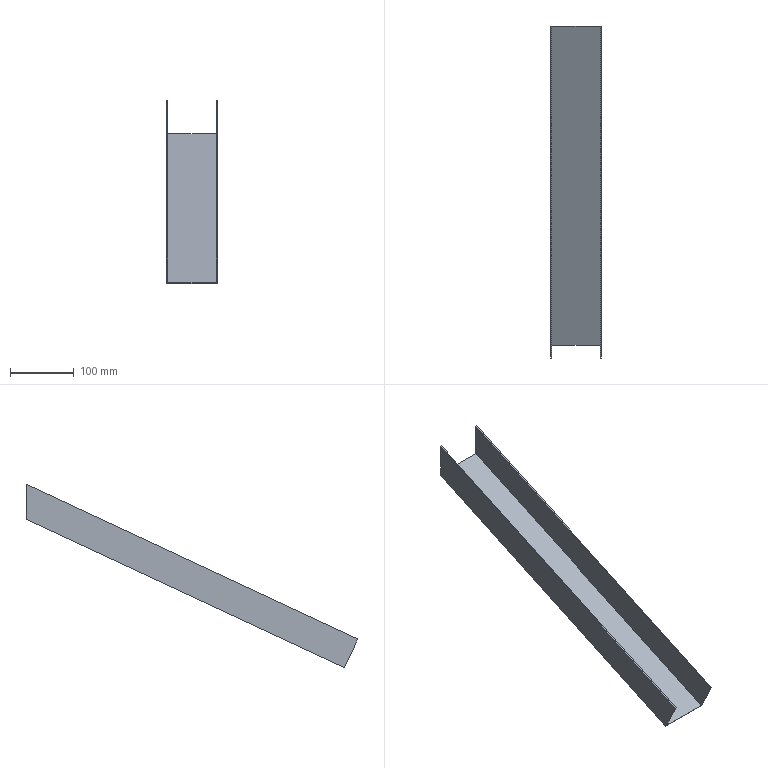Part | NX | features solid 2 | 1 solid | 10 faces | box 80 x 521.131 x 288.323 mm | volume 196597 mm3 | plane 10
STEP:
#1=CARTESIAN_POINT('',(400.,-525.,-154.948));
#2=VERTEX_POINT('',#1);
#3=CARTESIAN_POINT('',(402.,-525.,-154.948));
#4=VERTEX_POINT('',#3);
#5=CARTESIAN_POINT('',(400.,-525.,-154.948));
#6=DIRECTION('',(1.,0.,0.));
#7=VECTOR('',#6,1000.);
#8=LINE('',#5,#7);
#9=EDGE_CURVE('',#2,#4,#8,.T.);
#10=ORIENTED_EDGE('',*,*,#9,.T.);
#11=CARTESIAN_POINT('',(402.,-525.,-207.91));
#12=VERTEX_POINT('',#11);
#13=CARTESIAN_POINT('',(402.,-525.,-175.106));
#14=DIRECTION('',(0.,0.,-1.));
#15=VECTOR('',#14,1000.);
#16=LINE('',#13,#15);
#17=EDGE_CURVE('',#4,#12,#16,.T.);
#18=ORIENTED_EDGE('',*,*,#17,.T.);
#19=CARTESIAN_POINT('',(478.,-525.,-207.91));
#20=VERTEX_POINT('',#19);
#21=CARTESIAN_POINT('',(400.,-525.,-207.91));
#22=DIRECTION('',(1.,0.,0.));
#23=VECTOR('',#22,1000.);
#24=LINE('',#21,#23);
#25=EDGE_CURVE('',#12,#20,#24,.T.);
#26=ORIENTED_EDGE('',*,*,#25,.T.);
#27=CARTESIAN_POINT('',(478.,-525.,-154.948));
#28=VERTEX_POINT('',#27);
#29=CARTESIAN_POINT('',(478.,-525.,-215.));
#30=DIRECTION('',(0.,0.,-1.));
#31=VECTOR('',#30,1000.);
#32=LINE('',#29,#31);
#33=EDGE_CURVE('',#28,#20,#32,.T.);
#34=ORIENTED_EDGE('',*,*,#33,.F.);
#35=CARTESIAN_POINT('',(480.,-525.,-154.948));
#36=VERTEX_POINT('',#35);
#37=CARTESIAN_POINT('',(400.,-525.,-154.948));
#38=DIRECTION('',(1.,0.,0.));
#39=VECTOR('',#38,1000.);
#40=LINE('',#37,#39);
#41=EDGE_CURVE('',#28,#36,#40,.T.);
#42=ORIENTED_EDGE('',*,*,#41,.T.);
#43=CARTESIAN_POINT('',(480.,-525.,-210.116));
#44=VERTEX_POINT('',#43);
#45=CARTESIAN_POINT('',(480.,-525.,-215.));
#46=DIRECTION('',(0.,0.,-1.));
#47=VECTOR('',#46,1000.);
#48=LINE('',#45,#47);
#49=EDGE_CURVE('',#36,#44,#48,.T.);
#50=ORIENTED_EDGE('',*,*,#49,.T.);
#51=CARTESIAN_POINT('',(400.,-525.,-210.116));
#52=VERTEX_POINT('',#51);
#53=CARTESIAN_POINT('',(400.,-525.,-210.116));
#54=DIRECTION('',(1.,0.,0.));
#55=VECTOR('',#54,1000.);
#56=LINE('',#53,#55);
#57=EDGE_CURVE('',#52,#44,#56,.T.);
#58=ORIENTED_EDGE('',*,*,#57,.F.);
#59=CARTESIAN_POINT('',(400.,-525.,-175.106));
#60=DIRECTION('',(0.,0.,-1.));
#61=VECTOR('',#60,1000.);
#62=LINE('',#59,#61);
#63=EDGE_CURVE('',#2,#52,#62,.T.);
#64=ORIENTED_EDGE('',*,*,#63,.F.);
#65=EDGE_LOOP('',(#10,#18,#26,#34,#42,#50,#58,#64));
#66=FACE_BOUND('',#65,.T.);
#67=CARTESIAN_POINT('',(-1120.,-525.,-215.));
#68=DIRECTION('',(0.,1.,0.));
#69=DIRECTION('',(-1.,0.,0.));
#70=AXIS2_PLACEMENT_3D('',#67,#68,#69);
#71=PLANE('',#70);
#72=ADVANCED_FACE('',(#66),#71,.T.);
#73=CARTESIAN_POINT('',(480.,-1046.131,-397.955));
#74=VERTEX_POINT('',#73);
#75=CARTESIAN_POINT('',(478.,-1046.131,-397.955));
#76=VERTEX_POINT('',#75);
#77=CARTESIAN_POINT('',(400.,-1046.131,-397.955));
#78=DIRECTION('',(-1.,0.,0.));
#79=VECTOR('',#78,1000.);
#80=LINE('',#77,#79);
#81=EDGE_CURVE('',#74,#76,#80,.T.);
#82=ORIENTED_EDGE('',*,*,#81,.T.);
#83=CARTESIAN_POINT('',(478.,-1025.845,-441.458));
#84=VERTEX_POINT('',#83);
#85=CARTESIAN_POINT('',(478.,-1046.131,-397.955));
#86=DIRECTION('',(0.,0.4226,-0.9063));
#87=VECTOR('',#86,1000.);
#88=LINE('',#85,#87);
#89=EDGE_CURVE('',#76,#84,#88,.T.);
#90=ORIENTED_EDGE('',*,*,#89,.T.);
#91=CARTESIAN_POINT('',(402.,-1025.845,-441.458));
#92=VERTEX_POINT('',#91);
#93=CARTESIAN_POINT('',(400.,-1025.845,-441.458));
#94=DIRECTION('',(-1.,0.,0.));
#95=VECTOR('',#94,1000.);
#96=LINE('',#93,#95);
#97=EDGE_CURVE('',#84,#92,#96,.T.);
#98=ORIENTED_EDGE('',*,*,#97,.T.);
#99=CARTESIAN_POINT('',(402.,-1046.131,-397.955));
#100=VERTEX_POINT('',#99);
#101=CARTESIAN_POINT('',(402.,-1046.131,-397.955));
#102=DIRECTION('',(0.,0.4226,-0.9063));
#103=VECTOR('',#102,1000.);
#104=LINE('',#101,#103);
#105=EDGE_CURVE('',#100,#92,#104,.T.);
#106=ORIENTED_EDGE('',*,*,#105,.F.);
#107=CARTESIAN_POINT('',(400.,-1046.131,-397.955));
#108=VERTEX_POINT('',#107);
#109=CARTESIAN_POINT('',(400.,-1046.131,-397.955));
#110=DIRECTION('',(-1.,0.,0.));
#111=VECTOR('',#110,1000.);
#112=LINE('',#109,#111);
#113=EDGE_CURVE('',#100,#108,#112,.T.);
#114=ORIENTED_EDGE('',*,*,#113,.T.);
#115=CARTESIAN_POINT('',(400.,-1025.,-443.27));
#116=VERTEX_POINT('',#115);
#117=CARTESIAN_POINT('',(400.,-1046.131,-397.955));
#118=DIRECTION('',(0.,0.4226,-0.9063));
#119=VECTOR('',#118,1000.);
#120=LINE('',#117,#119);
#121=EDGE_CURVE('',#108,#116,#120,.T.);
#122=ORIENTED_EDGE('',*,*,#121,.T.);
#123=CARTESIAN_POINT('',(480.,-1025.,-443.27));
#124=VERTEX_POINT('',#123);
#125=CARTESIAN_POINT('',(400.,-1025.,-443.27));
#126=DIRECTION('',(-1.,0.,0.));
#127=VECTOR('',#126,1000.);
#128=LINE('',#125,#127);
#129=EDGE_CURVE('',#124,#116,#128,.T.);
#130=ORIENTED_EDGE('',*,*,#129,.F.);
#131=CARTESIAN_POINT('',(480.,-1046.131,-397.955));
#132=DIRECTION('',(0.,0.4226,-0.9063));
#133=VECTOR('',#132,1000.);
#134=LINE('',#131,#133);
#135=EDGE_CURVE('',#74,#124,#134,.T.);
#136=ORIENTED_EDGE('',*,*,#135,.F.);
#137=EDGE_LOOP('',(#82,#90,#98,#106,#114,#122,#130,#136));
#138=FACE_BOUND('',#137,.T.);
#139=CARTESIAN_POINT('',(400.,-1046.131,-397.955));
#140=DIRECTION('',(0.,-0.9063,-0.4226));
#141=DIRECTION('',(0.,0.4226,-0.9063));
#142=AXIS2_PLACEMENT_3D('',#139,#140,#141);
#143=PLANE('',#142);
#144=ADVANCED_FACE('',(#138),#143,.T.);
#145=ORIENTED_EDGE('',*,*,#113,.F.);
#146=CARTESIAN_POINT('',(402.,-568.231,-175.106));
#147=DIRECTION('',(0.,0.9063,0.4226));
#148=VECTOR('',#147,1000.);
#149=LINE('',#146,#148);
#150=EDGE_CURVE('',#100,#4,#149,.T.);
#151=ORIENTED_EDGE('',*,*,#150,.T.);
#152=ORIENTED_EDGE('',*,*,#9,.F.);
#153=CARTESIAN_POINT('',(400.,-568.231,-175.106));
#154=DIRECTION('',(0.,0.9063,0.4226));
#155=VECTOR('',#154,1000.);
#156=LINE('',#153,#155);
#157=EDGE_CURVE('',#108,#2,#156,.T.);
#158=ORIENTED_EDGE('',*,*,#157,.F.);
#159=EDGE_LOOP('',(#145,#151,#152,#158));
#160=FACE_BOUND('',#159,.T.);
#161=CARTESIAN_POINT('',(400.,-568.231,-175.106));
#162=DIRECTION('',(0.,0.4226,-0.9063));
#163=DIRECTION('',(-1.,0.,0.));
#164=AXIS2_PLACEMENT_3D('',#161,#162,#163);
#165=PLANE('',#164);
#166=ADVANCED_FACE('',(#160),#165,.F.);
#167=CARTESIAN_POINT('',(400.,-547.1,-220.422));
#168=DIRECTION('',(0.,0.9063,0.4226));
#169=VECTOR('',#168,1000.);
#170=LINE('',#167,#169);
#171=EDGE_CURVE('',#116,#52,#170,.T.);
#172=ORIENTED_EDGE('',*,*,#171,.F.);
#173=ORIENTED_EDGE('',*,*,#121,.F.);
#174=ORIENTED_EDGE('',*,*,#157,.T.);
#175=ORIENTED_EDGE('',*,*,#63,.T.);
#176=EDGE_LOOP('',(#172,#173,#174,#175));
#177=FACE_BOUND('',#176,.T.);
#178=CARTESIAN_POINT('',(400.,-568.231,-175.106));
#179=DIRECTION('',(-1.,0.,0.));
#180=DIRECTION('',(0.,0.,1.));
#181=AXIS2_PLACEMENT_3D('',#178,#179,#180);
#182=PLANE('',#181);
#183=ADVANCED_FACE('',(#177),#182,.T.);
#184=CARTESIAN_POINT('',(480.,-547.1,-220.422));
#185=DIRECTION('',(0.,-0.9063,-0.4226));
#186=VECTOR('',#185,1000.);
#187=LINE('',#184,#186);
#188=EDGE_CURVE('',#44,#124,#187,.T.);
#189=ORIENTED_EDGE('',*,*,#188,.F.);
#190=ORIENTED_EDGE('',*,*,#49,.F.);
#191=CARTESIAN_POINT('',(480.,-568.231,-175.106));
#192=DIRECTION('',(0.,-0.9063,-0.4226));
#193=VECTOR('',#192,1000.);
#194=LINE('',#191,#193);
#195=EDGE_CURVE('',#36,#74,#194,.T.);
#196=ORIENTED_EDGE('',*,*,#195,.T.);
#197=ORIENTED_EDGE('',*,*,#135,.T.);
#198=EDGE_LOOP('',(#189,#190,#196,#197));
#199=FACE_BOUND('',#198,.T.);
#200=CARTESIAN_POINT('',(480.,-568.231,-175.106));
#201=DIRECTION('',(1.,0.,0.));
#202=DIRECTION('',(0.,0.,-1.));
#203=AXIS2_PLACEMENT_3D('',#200,#201,#202);
#204=PLANE('',#203);
#205=ADVANCED_FACE('',(#199),#204,.T.);
#206=ORIENTED_EDGE('',*,*,#41,.F.);
#207=CARTESIAN_POINT('',(478.,-568.231,-175.106));
#208=DIRECTION('',(0.,-0.9063,-0.4226));
#209=VECTOR('',#208,1000.);
#210=LINE('',#207,#209);
#211=EDGE_CURVE('',#28,#76,#210,.T.);
#212=ORIENTED_EDGE('',*,*,#211,.T.);
#213=ORIENTED_EDGE('',*,*,#81,.F.);
#214=ORIENTED_EDGE('',*,*,#195,.F.);
#215=EDGE_LOOP('',(#206,#212,#213,#214));
#216=FACE_BOUND('',#215,.T.);
#217=CARTESIAN_POINT('',(400.,-568.231,-175.106));
#218=DIRECTION('',(0.,0.4226,-0.9063));
#219=DIRECTION('',(-1.,0.,0.));
#220=AXIS2_PLACEMENT_3D('',#217,#218,#219);
#221=PLANE('',#220);
#222=ADVANCED_FACE('',(#216),#221,.F.);
#223=ORIENTED_EDGE('',*,*,#171,.T.);
#224=ORIENTED_EDGE('',*,*,#57,.T.);
#225=ORIENTED_EDGE('',*,*,#188,.T.);
#226=ORIENTED_EDGE('',*,*,#129,.T.);
#227=EDGE_LOOP('',(#223,#224,#225,#226));
#228=FACE_BOUND('',#227,.T.);
#229=CARTESIAN_POINT('',(400.,-547.1,-220.422));
#230=DIRECTION('',(0.,0.4226,-0.9063));
#231=DIRECTION('',(-1.,0.,0.));
#232=AXIS2_PLACEMENT_3D('',#229,#230,#231);
#233=PLANE('',#232);
#234=ADVANCED_FACE('',(#228),#233,.T.);
#235=CARTESIAN_POINT('',(402.,-547.945,-218.609));
#236=DIRECTION('',(0.,0.9063,0.4226));
#237=VECTOR('',#236,1000.);
#238=LINE('',#235,#237);
#239=EDGE_CURVE('',#92,#12,#238,.T.);
#240=ORIENTED_EDGE('',*,*,#239,.T.);
#241=ORIENTED_EDGE('',*,*,#17,.F.);
#242=ORIENTED_EDGE('',*,*,#150,.F.);
#243=ORIENTED_EDGE('',*,*,#105,.T.);
#244=EDGE_LOOP('',(#240,#241,#242,#243));
#245=FACE_BOUND('',#244,.T.);
#246=CARTESIAN_POINT('',(402.,-568.231,-175.106));
#247=DIRECTION('',(-1.,0.,0.));
#248=DIRECTION('',(0.,0.,1.));
#249=AXIS2_PLACEMENT_3D('',#246,#247,#248);
#250=PLANE('',#249);
#251=ADVANCED_FACE('',(#245),#250,.F.);
#252=CARTESIAN_POINT('',(478.,-547.945,-218.609));
#253=DIRECTION('',(0.,-0.9063,-0.4226));
#254=VECTOR('',#253,1000.);
#255=LINE('',#252,#254);
#256=EDGE_CURVE('',#20,#84,#255,.T.);
#257=ORIENTED_EDGE('',*,*,#256,.T.);
#258=ORIENTED_EDGE('',*,*,#89,.F.);
#259=ORIENTED_EDGE('',*,*,#211,.F.);
#260=ORIENTED_EDGE('',*,*,#33,.T.);
#261=EDGE_LOOP('',(#257,#258,#259,#260));
#262=FACE_BOUND('',#261,.T.);
#263=CARTESIAN_POINT('',(478.,-568.231,-175.106));
#264=DIRECTION('',(1.,0.,0.));
#265=DIRECTION('',(0.,0.,-1.));
#266=AXIS2_PLACEMENT_3D('',#263,#264,#265);
#267=PLANE('',#266);
#268=ADVANCED_FACE('',(#262),#267,.F.);
#269=ORIENTED_EDGE('',*,*,#239,.F.);
#270=ORIENTED_EDGE('',*,*,#97,.F.);
#271=ORIENTED_EDGE('',*,*,#256,.F.);
#272=ORIENTED_EDGE('',*,*,#25,.F.);
#273=EDGE_LOOP('',(#269,#270,#271,#272));
#274=FACE_BOUND('',#273,.T.);
#275=CARTESIAN_POINT('',(400.,-547.945,-218.609));
#276=DIRECTION('',(0.,0.4226,-0.9063));
#277=DIRECTION('',(-1.,0.,0.));
#278=AXIS2_PLACEMENT_3D('',#275,#276,#277);
#279=PLANE('',#278);
#280=ADVANCED_FACE('',(#274),#279,.F.);
#281=CLOSED_SHELL('',(#72,#144,#166,#183,#205,#222,#234,#251,#268,#280));
#282=MANIFOLD_SOLID_BREP('',#281);
#283=(LENGTH_UNIT()NAMED_UNIT(*)SI_UNIT(.MILLI.,.METRE.));
#284=UNCERTAINTY_MEASURE_WITH_UNIT(LENGTH_MEASURE(0.00001),#283,'','');
#285=(NAMED_UNIT(*)PLANE_ANGLE_UNIT()SI_UNIT($,.RADIAN.));
#286=(NAMED_UNIT(*)SI_UNIT($,.STERADIAN.)SOLID_ANGLE_UNIT());
#287=(GEOMETRIC_REPRESENTATION_CONTEXT(3)GLOBAL_UNCERTAINTY_ASSIGNED_CONTEXT((#284))GLOBAL_UNIT_ASSIGNED_CONTEXT((#283,#285,#286))REPRESENTATION_CONTEXT('',''));
#288=ADVANCED_BREP_SHAPE_REPRESENTATION('',(#282),#287);